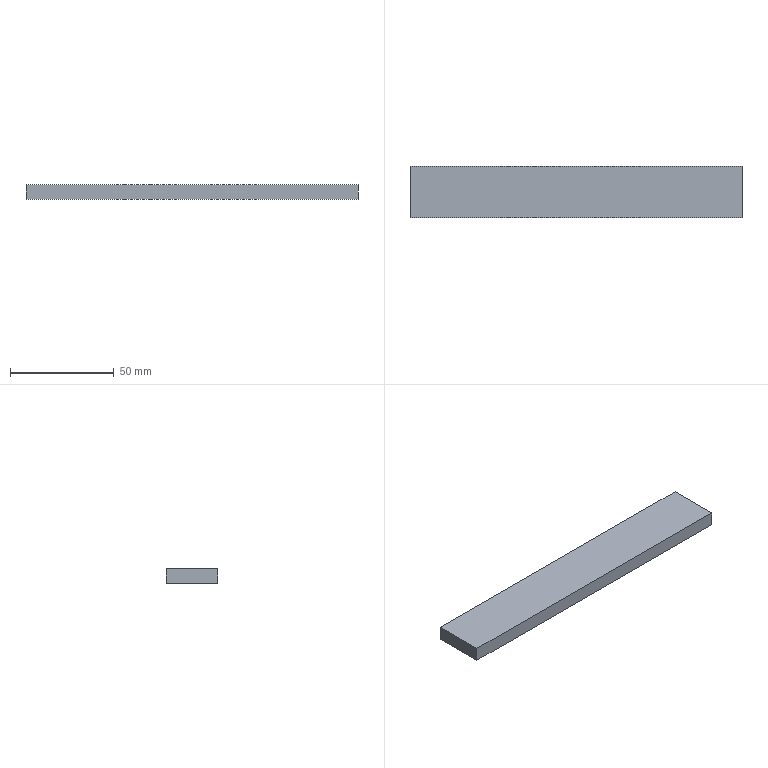Part | SolidWorks | features Extrusion 1 | 1 solid | 6 faces | box 160 x 25 x 7 mm | volume 28000 mm3 | plane 6
STEP:
#1=CARTESIAN_POINT('',(80.,-12.5,0.));
#2=VERTEX_POINT('',#1);
#3=CARTESIAN_POINT('',(80.,12.5,0.));
#4=VERTEX_POINT('',#3);
#5=CARTESIAN_POINT('',(80.,-12.5,0.));
#6=DIRECTION('',(0.,1.,0.));
#7=VECTOR('',#6,1000.);
#8=LINE('',#5,#7);
#9=EDGE_CURVE('',#2,#4,#8,.T.);
#10=ORIENTED_EDGE('',*,*,#9,.T.);
#11=CARTESIAN_POINT('',(80.,12.5,7.));
#12=VERTEX_POINT('',#11);
#13=CARTESIAN_POINT('',(80.,12.5,7.));
#14=DIRECTION('',(0.,0.,-1.));
#15=VECTOR('',#14,1000.);
#16=LINE('',#13,#15);
#17=EDGE_CURVE('',#12,#4,#16,.T.);
#18=ORIENTED_EDGE('',*,*,#17,.F.);
#19=CARTESIAN_POINT('',(80.,-12.5,7.));
#20=VERTEX_POINT('',#19);
#21=CARTESIAN_POINT('',(80.,-12.5,7.));
#22=DIRECTION('',(0.,1.,0.));
#23=VECTOR('',#22,1000.);
#24=LINE('',#21,#23);
#25=EDGE_CURVE('',#20,#12,#24,.T.);
#26=ORIENTED_EDGE('',*,*,#25,.F.);
#27=CARTESIAN_POINT('',(80.,-12.5,7.));
#28=DIRECTION('',(0.,0.,-1.));
#29=VECTOR('',#28,1000.);
#30=LINE('',#27,#29);
#31=EDGE_CURVE('',#20,#2,#30,.T.);
#32=ORIENTED_EDGE('',*,*,#31,.T.);
#33=EDGE_LOOP('',(#10,#18,#26,#32));
#34=FACE_OUTER_BOUND('',#33,.T.);
#35=CARTESIAN_POINT('',(80.,-12.5,7.));
#36=DIRECTION('',(-1.,0.,0.));
#37=DIRECTION('',(0.,0.,1.));
#38=AXIS2_PLACEMENT_3D('',#35,#36,#37);
#39=PLANE('',#38);
#40=ADVANCED_FACE('',(#34),#39,.F.);
#41=CARTESIAN_POINT('',(-80.,12.5,0.));
#42=VERTEX_POINT('',#41);
#43=CARTESIAN_POINT('',(-80.,12.5,0.));
#44=DIRECTION('',(-1.,0.,0.));
#45=VECTOR('',#44,1000.);
#46=LINE('',#43,#45);
#47=EDGE_CURVE('',#4,#42,#46,.T.);
#48=ORIENTED_EDGE('',*,*,#47,.T.);
#49=CARTESIAN_POINT('',(-80.,12.5,7.));
#50=VERTEX_POINT('',#49);
#51=CARTESIAN_POINT('',(-80.,12.5,7.));
#52=DIRECTION('',(0.,0.,-1.));
#53=VECTOR('',#52,1000.);
#54=LINE('',#51,#53);
#55=EDGE_CURVE('',#50,#42,#54,.T.);
#56=ORIENTED_EDGE('',*,*,#55,.F.);
#57=CARTESIAN_POINT('',(-80.,12.5,7.));
#58=DIRECTION('',(-1.,0.,0.));
#59=VECTOR('',#58,1000.);
#60=LINE('',#57,#59);
#61=EDGE_CURVE('',#12,#50,#60,.T.);
#62=ORIENTED_EDGE('',*,*,#61,.F.);
#63=ORIENTED_EDGE('',*,*,#17,.T.);
#64=EDGE_LOOP('',(#48,#56,#62,#63));
#65=FACE_OUTER_BOUND('',#64,.T.);
#66=CARTESIAN_POINT('',(-80.,12.5,7.));
#67=DIRECTION('',(0.,-1.,0.));
#68=DIRECTION('',(0.,0.,-1.));
#69=AXIS2_PLACEMENT_3D('',#66,#67,#68);
#70=PLANE('',#69);
#71=ADVANCED_FACE('',(#65),#70,.F.);
#72=CARTESIAN_POINT('',(-80.,-12.5,0.));
#73=VERTEX_POINT('',#72);
#74=CARTESIAN_POINT('',(-80.,-12.5,0.));
#75=DIRECTION('',(0.,-1.,0.));
#76=VECTOR('',#75,1000.);
#77=LINE('',#74,#76);
#78=EDGE_CURVE('',#42,#73,#77,.T.);
#79=ORIENTED_EDGE('',*,*,#78,.T.);
#80=CARTESIAN_POINT('',(-80.,-12.5,7.));
#81=VERTEX_POINT('',#80);
#82=CARTESIAN_POINT('',(-80.,-12.5,7.));
#83=DIRECTION('',(0.,0.,-1.));
#84=VECTOR('',#83,1000.);
#85=LINE('',#82,#84);
#86=EDGE_CURVE('',#81,#73,#85,.T.);
#87=ORIENTED_EDGE('',*,*,#86,.F.);
#88=CARTESIAN_POINT('',(-80.,-12.5,7.));
#89=DIRECTION('',(0.,-1.,0.));
#90=VECTOR('',#89,1000.);
#91=LINE('',#88,#90);
#92=EDGE_CURVE('',#50,#81,#91,.T.);
#93=ORIENTED_EDGE('',*,*,#92,.F.);
#94=ORIENTED_EDGE('',*,*,#55,.T.);
#95=EDGE_LOOP('',(#79,#87,#93,#94));
#96=FACE_OUTER_BOUND('',#95,.T.);
#97=CARTESIAN_POINT('',(-80.,-12.5,7.));
#98=DIRECTION('',(1.,0.,0.));
#99=DIRECTION('',(0.,0.,-1.));
#100=AXIS2_PLACEMENT_3D('',#97,#98,#99);
#101=PLANE('',#100);
#102=ADVANCED_FACE('',(#96),#101,.F.);
#103=CARTESIAN_POINT('',(-80.,-12.5,0.));
#104=DIRECTION('',(1.,0.,0.));
#105=VECTOR('',#104,1000.);
#106=LINE('',#103,#105);
#107=EDGE_CURVE('',#73,#2,#106,.T.);
#108=ORIENTED_EDGE('',*,*,#107,.T.);
#109=ORIENTED_EDGE('',*,*,#31,.F.);
#110=CARTESIAN_POINT('',(-80.,-12.5,7.));
#111=DIRECTION('',(1.,0.,0.));
#112=VECTOR('',#111,1000.);
#113=LINE('',#110,#112);
#114=EDGE_CURVE('',#81,#20,#113,.T.);
#115=ORIENTED_EDGE('',*,*,#114,.F.);
#116=ORIENTED_EDGE('',*,*,#86,.T.);
#117=EDGE_LOOP('',(#108,#109,#115,#116));
#118=FACE_OUTER_BOUND('',#117,.T.);
#119=CARTESIAN_POINT('',(-80.,-12.5,7.));
#120=DIRECTION('',(0.,1.,0.));
#121=DIRECTION('',(0.,0.,1.));
#122=AXIS2_PLACEMENT_3D('',#119,#120,#121);
#123=PLANE('',#122);
#124=ADVANCED_FACE('',(#118),#123,.F.);
#125=ORIENTED_EDGE('',*,*,#25,.T.);
#126=ORIENTED_EDGE('',*,*,#61,.T.);
#127=ORIENTED_EDGE('',*,*,#92,.T.);
#128=ORIENTED_EDGE('',*,*,#114,.T.);
#129=EDGE_LOOP('',(#125,#126,#127,#128));
#130=FACE_OUTER_BOUND('',#129,.T.);
#131=CARTESIAN_POINT('',(0.,0.,7.));
#132=DIRECTION('',(0.,0.,-1.));
#133=DIRECTION('',(-1.,0.,0.));
#134=AXIS2_PLACEMENT_3D('',#131,#132,#133);
#135=PLANE('',#134);
#136=ADVANCED_FACE('',(#130),#135,.F.);
#137=ORIENTED_EDGE('',*,*,#9,.F.);
#138=ORIENTED_EDGE('',*,*,#107,.F.);
#139=ORIENTED_EDGE('',*,*,#78,.F.);
#140=ORIENTED_EDGE('',*,*,#47,.F.);
#141=EDGE_LOOP('',(#137,#138,#139,#140));
#142=FACE_OUTER_BOUND('',#141,.T.);
#143=CARTESIAN_POINT('',(0.,0.,0.));
#144=DIRECTION('',(0.,0.,-1.));
#145=DIRECTION('',(-1.,0.,0.));
#146=AXIS2_PLACEMENT_3D('',#143,#144,#145);
#147=PLANE('',#146);
#148=ADVANCED_FACE('',(#142),#147,.T.);
#149=CLOSED_SHELL('',(#40,#71,#102,#124,#136,#148));
#150=MANIFOLD_SOLID_BREP('',#149);
#151=CARTESIAN_POINT('',(0.,0.,0.));
#152=DIRECTION('',(0.,0.,1.));
#153=DIRECTION('',(1.,0.,0.));
#154=AXIS2_PLACEMENT_3D('',#151,#152,#153);
#155=(LENGTH_UNIT()NAMED_UNIT(*)SI_UNIT(.MILLI.,.METRE.));
#156=UNCERTAINTY_MEASURE_WITH_UNIT(LENGTH_MEASURE(0.00001),#155,'','');
#157=(NAMED_UNIT(*)PLANE_ANGLE_UNIT()SI_UNIT($,.RADIAN.));
#158=(NAMED_UNIT(*)SI_UNIT($,.STERADIAN.)SOLID_ANGLE_UNIT());
#159=(GEOMETRIC_REPRESENTATION_CONTEXT(3)GLOBAL_UNCERTAINTY_ASSIGNED_CONTEXT((#156))GLOBAL_UNIT_ASSIGNED_CONTEXT((#155,#157,#158))REPRESENTATION_CONTEXT('',''));
#160=ADVANCED_BREP_SHAPE_REPRESENTATION('',(#150,#154),#159);